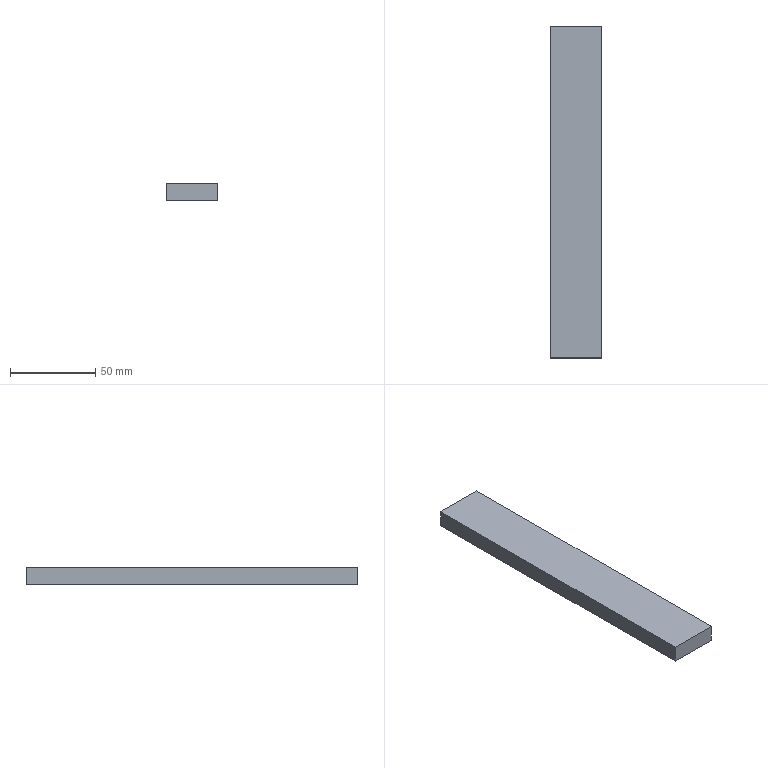Part | NX | features solid 2 | 1 solid | 6 faces | box 30 x 195 x 10 mm | volume 58500 mm3 | plane 6
STEP:
#1=CARTESIAN_POINT('',(-509.173,295.,-10.));
#2=VERTEX_POINT('',#1);
#3=CARTESIAN_POINT('',(-479.173,295.,-10.));
#4=VERTEX_POINT('',#3);
#5=CARTESIAN_POINT('',(-374.173,295.,-10.));
#6=DIRECTION('',(1.,0.,0.));
#7=VECTOR('',#6,1000.);
#8=LINE('',#5,#7);
#9=EDGE_CURVE('',#2,#4,#8,.T.);
#10=ORIENTED_EDGE('',*,*,#9,.F.);
#11=CARTESIAN_POINT('',(-509.173,295.,-20.));
#12=VERTEX_POINT('',#11);
#13=CARTESIAN_POINT('',(-509.173,295.,20.));
#14=DIRECTION('',(0.,0.,-1.));
#15=VECTOR('',#14,1000.);
#16=LINE('',#13,#15);
#17=EDGE_CURVE('',#2,#12,#16,.T.);
#18=ORIENTED_EDGE('',*,*,#17,.T.);
#19=CARTESIAN_POINT('',(-479.173,295.,-20.));
#20=VERTEX_POINT('',#19);
#21=CARTESIAN_POINT('',(-374.173,295.,-20.));
#22=DIRECTION('',(1.,0.,0.));
#23=VECTOR('',#22,1000.);
#24=LINE('',#21,#23);
#25=EDGE_CURVE('',#12,#20,#24,.T.);
#26=ORIENTED_EDGE('',*,*,#25,.T.);
#27=CARTESIAN_POINT('',(-479.173,295.,20.));
#28=DIRECTION('',(0.,0.,-1.));
#29=VECTOR('',#28,1000.);
#30=LINE('',#27,#29);
#31=EDGE_CURVE('',#4,#20,#30,.T.);
#32=ORIENTED_EDGE('',*,*,#31,.F.);
#33=EDGE_LOOP('',(#10,#18,#26,#32));
#34=FACE_BOUND('',#33,.T.);
#35=CARTESIAN_POINT('',(-509.173,295.,20.));
#36=DIRECTION('',(0.,-1.,0.));
#37=DIRECTION('',(0.,0.,-1.));
#38=AXIS2_PLACEMENT_3D('',#35,#36,#37);
#39=PLANE('',#38);
#40=ADVANCED_FACE('',(#34),#39,.T.);
#41=CARTESIAN_POINT('',(-479.173,490.,-10.));
#42=VERTEX_POINT('',#41);
#43=CARTESIAN_POINT('',(-479.173,490.,-20.));
#44=VERTEX_POINT('',#43);
#45=CARTESIAN_POINT('',(-479.173,490.,-10.));
#46=DIRECTION('',(0.,0.,-1.));
#47=VECTOR('',#46,1000.);
#48=LINE('',#45,#47);
#49=EDGE_CURVE('',#42,#44,#48,.T.);
#50=ORIENTED_EDGE('',*,*,#49,.F.);
#51=CARTESIAN_POINT('',(-479.173,460.,-10.));
#52=DIRECTION('',(0.,-1.,0.));
#53=VECTOR('',#52,1000.);
#54=LINE('',#51,#53);
#55=EDGE_CURVE('',#42,#4,#54,.T.);
#56=ORIENTED_EDGE('',*,*,#55,.T.);
#57=ORIENTED_EDGE('',*,*,#31,.T.);
#58=CARTESIAN_POINT('',(-479.173,490.,-20.));
#59=DIRECTION('',(0.,1.,0.));
#60=VECTOR('',#59,1000.);
#61=LINE('',#58,#60);
#62=EDGE_CURVE('',#44,#20,#61,.F.);
#63=ORIENTED_EDGE('',*,*,#62,.F.);
#64=EDGE_LOOP('',(#50,#56,#57,#63));
#65=FACE_BOUND('',#64,.T.);
#66=CARTESIAN_POINT('',(-479.173,490.,0.));
#67=DIRECTION('',(-1.,0.,0.));
#68=DIRECTION('',(0.,0.,1.));
#69=AXIS2_PLACEMENT_3D('',#66,#67,#68);
#70=PLANE('',#69);
#71=ADVANCED_FACE('',(#65),#70,.F.);
#72=CARTESIAN_POINT('',(-509.173,490.,-20.));
#73=VERTEX_POINT('',#72);
#74=CARTESIAN_POINT('',(-509.173,490.,-10.));
#75=VERTEX_POINT('',#74);
#76=CARTESIAN_POINT('',(-509.173,490.,0.));
#77=DIRECTION('',(0.,0.,1.));
#78=VECTOR('',#77,1000.);
#79=LINE('',#76,#78);
#80=EDGE_CURVE('',#73,#75,#79,.T.);
#81=ORIENTED_EDGE('',*,*,#80,.F.);
#82=CARTESIAN_POINT('',(-509.173,490.,-20.));
#83=DIRECTION('',(0.,1.,0.));
#84=VECTOR('',#83,1000.);
#85=LINE('',#82,#84);
#86=EDGE_CURVE('',#73,#12,#85,.F.);
#87=ORIENTED_EDGE('',*,*,#86,.T.);
#88=ORIENTED_EDGE('',*,*,#17,.F.);
#89=CARTESIAN_POINT('',(-509.173,460.,-10.));
#90=DIRECTION('',(0.,-1.,0.));
#91=VECTOR('',#90,1000.);
#92=LINE('',#89,#91);
#93=EDGE_CURVE('',#75,#2,#92,.T.);
#94=ORIENTED_EDGE('',*,*,#93,.F.);
#95=EDGE_LOOP('',(#81,#87,#88,#94));
#96=FACE_BOUND('',#95,.T.);
#97=CARTESIAN_POINT('',(-509.173,490.,0.));
#98=DIRECTION('',(-1.,0.,0.));
#99=DIRECTION('',(0.,0.,1.));
#100=AXIS2_PLACEMENT_3D('',#97,#98,#99);
#101=PLANE('',#100);
#102=ADVANCED_FACE('',(#96),#101,.T.);
#103=ORIENTED_EDGE('',*,*,#86,.F.);
#104=CARTESIAN_POINT('',(-374.173,490.,-20.));
#105=DIRECTION('',(1.,0.,0.));
#106=VECTOR('',#105,1000.);
#107=LINE('',#104,#106);
#108=EDGE_CURVE('',#73,#44,#107,.T.);
#109=ORIENTED_EDGE('',*,*,#108,.T.);
#110=ORIENTED_EDGE('',*,*,#62,.T.);
#111=ORIENTED_EDGE('',*,*,#25,.F.);
#112=EDGE_LOOP('',(#103,#109,#110,#111));
#113=FACE_BOUND('',#112,.T.);
#114=CARTESIAN_POINT('',(-374.173,460.,-20.));
#115=DIRECTION('',(0.,0.,1.));
#116=DIRECTION('',(1.,0.,0.));
#117=AXIS2_PLACEMENT_3D('',#114,#115,#116);
#118=PLANE('',#117);
#119=ADVANCED_FACE('',(#113),#118,.F.);
#120=CARTESIAN_POINT('',(-374.173,490.,-10.));
#121=DIRECTION('',(1.,0.,0.));
#122=VECTOR('',#121,1000.);
#123=LINE('',#120,#122);
#124=EDGE_CURVE('',#75,#42,#123,.T.);
#125=ORIENTED_EDGE('',*,*,#124,.F.);
#126=ORIENTED_EDGE('',*,*,#93,.T.);
#127=ORIENTED_EDGE('',*,*,#9,.T.);
#128=ORIENTED_EDGE('',*,*,#55,.F.);
#129=EDGE_LOOP('',(#125,#126,#127,#128));
#130=FACE_BOUND('',#129,.T.);
#131=CARTESIAN_POINT('',(-374.173,460.,-10.));
#132=DIRECTION('',(0.,0.,1.));
#133=DIRECTION('',(1.,0.,0.));
#134=AXIS2_PLACEMENT_3D('',#131,#132,#133);
#135=PLANE('',#134);
#136=ADVANCED_FACE('',(#130),#135,.T.);
#137=ORIENTED_EDGE('',*,*,#108,.F.);
#138=ORIENTED_EDGE('',*,*,#80,.T.);
#139=ORIENTED_EDGE('',*,*,#124,.T.);
#140=ORIENTED_EDGE('',*,*,#49,.T.);
#141=EDGE_LOOP('',(#137,#138,#139,#140));
#142=FACE_BOUND('',#141,.T.);
#143=CARTESIAN_POINT('',(-295.173,490.,-10.));
#144=DIRECTION('',(0.,-1.,0.));
#145=DIRECTION('',(1.,0.,0.));
#146=AXIS2_PLACEMENT_3D('',#143,#144,#145);
#147=PLANE('',#146);
#148=ADVANCED_FACE('',(#142),#147,.F.);
#149=CLOSED_SHELL('',(#40,#71,#102,#119,#136,#148));
#150=MANIFOLD_SOLID_BREP('',#149);
#151=(LENGTH_UNIT()NAMED_UNIT(*)SI_UNIT(.MILLI.,.METRE.));
#152=UNCERTAINTY_MEASURE_WITH_UNIT(LENGTH_MEASURE(0.00001),#151,'','');
#153=(NAMED_UNIT(*)PLANE_ANGLE_UNIT()SI_UNIT($,.RADIAN.));
#154=(NAMED_UNIT(*)SI_UNIT($,.STERADIAN.)SOLID_ANGLE_UNIT());
#155=(GEOMETRIC_REPRESENTATION_CONTEXT(3)GLOBAL_UNCERTAINTY_ASSIGNED_CONTEXT((#152))GLOBAL_UNIT_ASSIGNED_CONTEXT((#151,#153,#154))REPRESENTATION_CONTEXT('',''));
#156=ADVANCED_BREP_SHAPE_REPRESENTATION('',(#150),#155);